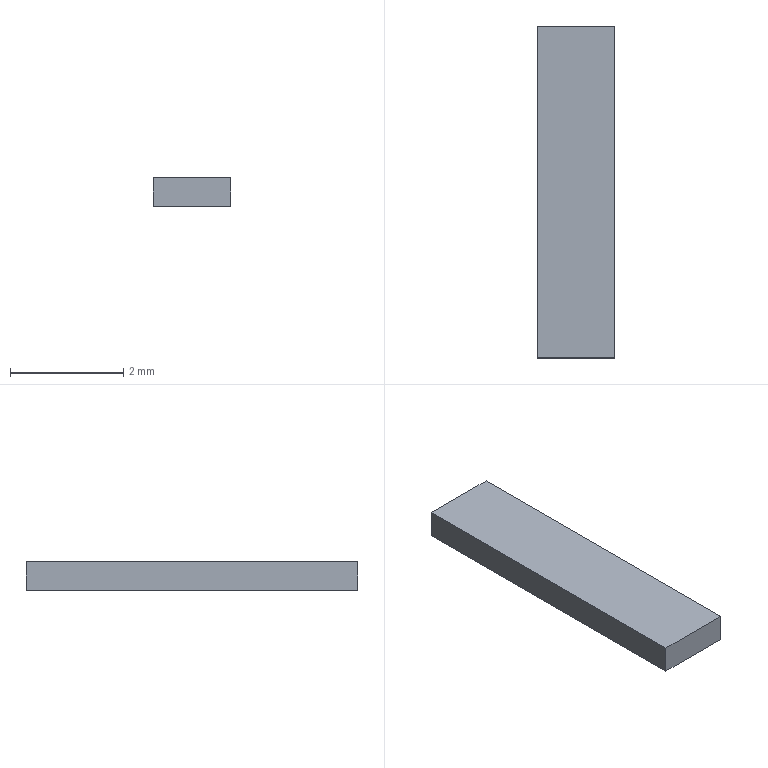Part | SolidWorks | features BaseBody 1 | 1 solid | 6 faces | box 1.375 x 5.875 x 0.5 mm | volume 4.039 mm3 | plane 6
STEP:
#1=CARTESIAN_POINT('',(-18.5,-14.625,1.));
#2=VERTEX_POINT('',#1);
#3=CARTESIAN_POINT('',(-18.5,-20.5,1.));
#4=VERTEX_POINT('',#3);
#5=CARTESIAN_POINT('',(-18.5,-14.625,1.));
#6=DIRECTION('',(0.,-1.,0.));
#7=VECTOR('',#6,1000.);
#8=LINE('',#5,#7);
#9=EDGE_CURVE('',#2,#4,#8,.T.);
#10=ORIENTED_EDGE('',*,*,#9,.T.);
#11=CARTESIAN_POINT('',(-18.5,-20.5,1.5));
#12=VERTEX_POINT('',#11);
#13=CARTESIAN_POINT('',(-18.5,-20.5,1.5));
#14=DIRECTION('',(0.,0.,-1.));
#15=VECTOR('',#14,1000.);
#16=LINE('',#13,#15);
#17=EDGE_CURVE('',#12,#4,#16,.T.);
#18=ORIENTED_EDGE('',*,*,#17,.F.);
#19=CARTESIAN_POINT('',(-18.5,-14.625,1.5));
#20=VERTEX_POINT('',#19);
#21=CARTESIAN_POINT('',(-18.5,-14.625,1.5));
#22=DIRECTION('',(0.,-1.,0.));
#23=VECTOR('',#22,1000.);
#24=LINE('',#21,#23);
#25=EDGE_CURVE('',#20,#12,#24,.T.);
#26=ORIENTED_EDGE('',*,*,#25,.F.);
#27=CARTESIAN_POINT('',(-18.5,-14.625,1.5));
#28=DIRECTION('',(0.,0.,-1.));
#29=VECTOR('',#28,1000.);
#30=LINE('',#27,#29);
#31=EDGE_CURVE('',#20,#2,#30,.T.);
#32=ORIENTED_EDGE('',*,*,#31,.T.);
#33=EDGE_LOOP('',(#10,#18,#26,#32));
#34=FACE_OUTER_BOUND('',#33,.T.);
#35=CARTESIAN_POINT('',(-18.5,-14.625,1.5));
#36=DIRECTION('',(1.,0.,0.));
#37=DIRECTION('',(0.,1.,0.));
#38=AXIS2_PLACEMENT_3D('',#35,#36,#37);
#39=PLANE('',#38);
#40=ADVANCED_FACE('',(#34),#39,.F.);
#41=CARTESIAN_POINT('',(-17.125,-20.5,1.));
#42=VERTEX_POINT('',#41);
#43=CARTESIAN_POINT('',(-18.5,-20.5,1.));
#44=DIRECTION('',(1.,0.,0.));
#45=VECTOR('',#44,1000.);
#46=LINE('',#43,#45);
#47=EDGE_CURVE('',#4,#42,#46,.T.);
#48=ORIENTED_EDGE('',*,*,#47,.T.);
#49=CARTESIAN_POINT('',(-17.125,-20.5,1.5));
#50=VERTEX_POINT('',#49);
#51=CARTESIAN_POINT('',(-17.125,-20.5,1.5));
#52=DIRECTION('',(0.,0.,-1.));
#53=VECTOR('',#52,1000.);
#54=LINE('',#51,#53);
#55=EDGE_CURVE('',#50,#42,#54,.T.);
#56=ORIENTED_EDGE('',*,*,#55,.F.);
#57=CARTESIAN_POINT('',(-18.5,-20.5,1.5));
#58=DIRECTION('',(1.,0.,0.));
#59=VECTOR('',#58,1000.);
#60=LINE('',#57,#59);
#61=EDGE_CURVE('',#12,#50,#60,.T.);
#62=ORIENTED_EDGE('',*,*,#61,.F.);
#63=ORIENTED_EDGE('',*,*,#17,.T.);
#64=EDGE_LOOP('',(#48,#56,#62,#63));
#65=FACE_OUTER_BOUND('',#64,.T.);
#66=CARTESIAN_POINT('',(-18.5,-20.5,1.5));
#67=DIRECTION('',(0.,1.,0.));
#68=DIRECTION('',(0.,0.,1.));
#69=AXIS2_PLACEMENT_3D('',#66,#67,#68);
#70=PLANE('',#69);
#71=ADVANCED_FACE('',(#65),#70,.F.);
#72=CARTESIAN_POINT('',(-17.125,-14.625,1.));
#73=VERTEX_POINT('',#72);
#74=CARTESIAN_POINT('',(-17.125,-20.5,1.));
#75=DIRECTION('',(0.,1.,0.));
#76=VECTOR('',#75,1000.);
#77=LINE('',#74,#76);
#78=EDGE_CURVE('',#42,#73,#77,.T.);
#79=ORIENTED_EDGE('',*,*,#78,.T.);
#80=CARTESIAN_POINT('',(-17.125,-14.625,1.5));
#81=VERTEX_POINT('',#80);
#82=CARTESIAN_POINT('',(-17.125,-14.625,1.5));
#83=DIRECTION('',(0.,0.,-1.));
#84=VECTOR('',#83,1000.);
#85=LINE('',#82,#84);
#86=EDGE_CURVE('',#81,#73,#85,.T.);
#87=ORIENTED_EDGE('',*,*,#86,.F.);
#88=CARTESIAN_POINT('',(-17.125,-20.5,1.5));
#89=DIRECTION('',(0.,1.,0.));
#90=VECTOR('',#89,1000.);
#91=LINE('',#88,#90);
#92=EDGE_CURVE('',#50,#81,#91,.T.);
#93=ORIENTED_EDGE('',*,*,#92,.F.);
#94=ORIENTED_EDGE('',*,*,#55,.T.);
#95=EDGE_LOOP('',(#79,#87,#93,#94));
#96=FACE_OUTER_BOUND('',#95,.T.);
#97=CARTESIAN_POINT('',(-17.125,-20.5,1.5));
#98=DIRECTION('',(-1.,0.,0.));
#99=DIRECTION('',(0.,0.,1.));
#100=AXIS2_PLACEMENT_3D('',#97,#98,#99);
#101=PLANE('',#100);
#102=ADVANCED_FACE('',(#96),#101,.F.);
#103=CARTESIAN_POINT('',(-17.125,-14.625,1.));
#104=DIRECTION('',(-1.,0.,0.));
#105=VECTOR('',#104,1000.);
#106=LINE('',#103,#105);
#107=EDGE_CURVE('',#73,#2,#106,.T.);
#108=ORIENTED_EDGE('',*,*,#107,.T.);
#109=ORIENTED_EDGE('',*,*,#31,.F.);
#110=CARTESIAN_POINT('',(-17.125,-14.625,1.5));
#111=DIRECTION('',(-1.,0.,0.));
#112=VECTOR('',#111,1000.);
#113=LINE('',#110,#112);
#114=EDGE_CURVE('',#81,#20,#113,.T.);
#115=ORIENTED_EDGE('',*,*,#114,.F.);
#116=ORIENTED_EDGE('',*,*,#86,.T.);
#117=EDGE_LOOP('',(#108,#109,#115,#116));
#118=FACE_OUTER_BOUND('',#117,.T.);
#119=CARTESIAN_POINT('',(-17.125,-14.625,1.5));
#120=DIRECTION('',(0.,-1.,0.));
#121=DIRECTION('',(0.,0.,-1.));
#122=AXIS2_PLACEMENT_3D('',#119,#120,#121);
#123=PLANE('',#122);
#124=ADVANCED_FACE('',(#118),#123,.F.);
#125=ORIENTED_EDGE('',*,*,#25,.T.);
#126=ORIENTED_EDGE('',*,*,#61,.T.);
#127=ORIENTED_EDGE('',*,*,#92,.T.);
#128=ORIENTED_EDGE('',*,*,#114,.T.);
#129=EDGE_LOOP('',(#125,#126,#127,#128));
#130=FACE_OUTER_BOUND('',#129,.T.);
#131=CARTESIAN_POINT('',(0.,0.,1.5));
#132=DIRECTION('',(0.,0.,1.));
#133=DIRECTION('',(1.,0.,0.));
#134=AXIS2_PLACEMENT_3D('',#131,#132,#133);
#135=PLANE('',#134);
#136=ADVANCED_FACE('',(#130),#135,.T.);
#137=ORIENTED_EDGE('',*,*,#9,.F.);
#138=ORIENTED_EDGE('',*,*,#107,.F.);
#139=ORIENTED_EDGE('',*,*,#78,.F.);
#140=ORIENTED_EDGE('',*,*,#47,.F.);
#141=EDGE_LOOP('',(#137,#138,#139,#140));
#142=FACE_OUTER_BOUND('',#141,.T.);
#143=CARTESIAN_POINT('',(0.,0.,1.));
#144=DIRECTION('',(0.,0.,1.));
#145=DIRECTION('',(1.,0.,0.));
#146=AXIS2_PLACEMENT_3D('',#143,#144,#145);
#147=PLANE('',#146);
#148=ADVANCED_FACE('',(#142),#147,.F.);
#149=CLOSED_SHELL('',(#40,#71,#102,#124,#136,#148));
#150=MANIFOLD_SOLID_BREP('',#149);
#151=CARTESIAN_POINT('',(0.,0.,0.));
#152=DIRECTION('',(0.,0.,1.));
#153=DIRECTION('',(1.,0.,0.));
#154=AXIS2_PLACEMENT_3D('',#151,#152,#153);
#155=(LENGTH_UNIT()NAMED_UNIT(*)SI_UNIT(.MILLI.,.METRE.));
#156=UNCERTAINTY_MEASURE_WITH_UNIT(LENGTH_MEASURE(0.00001),#155,'','');
#157=(NAMED_UNIT(*)PLANE_ANGLE_UNIT()SI_UNIT($,.RADIAN.));
#158=(NAMED_UNIT(*)SI_UNIT($,.STERADIAN.)SOLID_ANGLE_UNIT());
#159=(GEOMETRIC_REPRESENTATION_CONTEXT(3)GLOBAL_UNCERTAINTY_ASSIGNED_CONTEXT((#156))GLOBAL_UNIT_ASSIGNED_CONTEXT((#155,#157,#158))REPRESENTATION_CONTEXT('',''));
#160=ADVANCED_BREP_SHAPE_REPRESENTATION('',(#150,#154),#159);